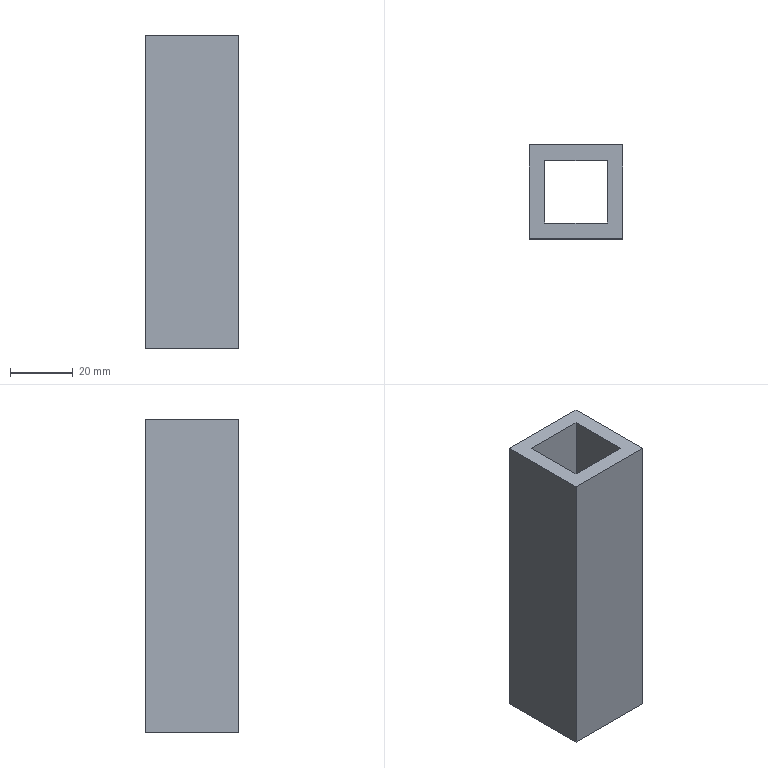Part | NX | features solid 2 | 1 solid | 10 faces | box 30 x 30 x 100 mm | volume 50000 mm3 | plane 10
STEP:
#1=CARTESIAN_POINT('',(-205.,215.,-80.));
#2=VERTEX_POINT('',#1);
#3=CARTESIAN_POINT('',(-175.,215.,-80.));
#4=VERTEX_POINT('',#3);
#5=CARTESIAN_POINT('',(-605.,215.,-80.));
#6=DIRECTION('',(-1.,0.,0.));
#7=VECTOR('',#6,1000.);
#8=LINE('',#5,#7);
#9=EDGE_CURVE('',#2,#4,#8,.F.);
#10=ORIENTED_EDGE('',*,*,#9,.F.);
#11=CARTESIAN_POINT('',(-205.,215.,-180.));
#12=VERTEX_POINT('',#11);
#13=CARTESIAN_POINT('',(-205.,215.,-125.));
#14=DIRECTION('',(0.,0.,1.));
#15=VECTOR('',#14,1000.);
#16=LINE('',#13,#15);
#17=EDGE_CURVE('',#2,#12,#16,.F.);
#18=ORIENTED_EDGE('',*,*,#17,.T.);
#19=CARTESIAN_POINT('',(-175.,215.,-180.));
#20=VERTEX_POINT('',#19);
#21=CARTESIAN_POINT('',(-605.,215.,-180.));
#22=DIRECTION('',(-1.,0.,0.));
#23=VECTOR('',#22,1000.);
#24=LINE('',#21,#23);
#25=EDGE_CURVE('',#20,#12,#24,.T.);
#26=ORIENTED_EDGE('',*,*,#25,.F.);
#27=CARTESIAN_POINT('',(-175.,215.,-125.));
#28=DIRECTION('',(0.,0.,1.));
#29=VECTOR('',#28,1000.);
#30=LINE('',#27,#29);
#31=EDGE_CURVE('',#4,#20,#30,.F.);
#32=ORIENTED_EDGE('',*,*,#31,.F.);
#33=EDGE_LOOP('',(#10,#18,#26,#32));
#34=FACE_BOUND('',#33,.T.);
#35=CARTESIAN_POINT('',(-605.,215.,-125.));
#36=DIRECTION('',(0.,1.,0.));
#37=DIRECTION('',(0.,0.,-1.));
#38=AXIS2_PLACEMENT_3D('',#35,#36,#37);
#39=PLANE('',#38);
#40=ADVANCED_FACE('',(#34),#39,.F.);
#41=CARTESIAN_POINT('',(-205.,245.,-80.));
#42=VERTEX_POINT('',#41);
#43=CARTESIAN_POINT('',(-205.,245.,-180.));
#44=VERTEX_POINT('',#43);
#45=CARTESIAN_POINT('',(-205.,245.,-125.));
#46=DIRECTION('',(0.,0.,1.));
#47=VECTOR('',#46,1000.);
#48=LINE('',#45,#47);
#49=EDGE_CURVE('',#42,#44,#48,.F.);
#50=ORIENTED_EDGE('',*,*,#49,.F.);
#51=CARTESIAN_POINT('',(-175.,245.,-80.));
#52=VERTEX_POINT('',#51);
#53=CARTESIAN_POINT('',(-605.,245.,-80.));
#54=DIRECTION('',(-1.,0.,0.));
#55=VECTOR('',#54,1000.);
#56=LINE('',#53,#55);
#57=EDGE_CURVE('',#42,#52,#56,.F.);
#58=ORIENTED_EDGE('',*,*,#57,.T.);
#59=CARTESIAN_POINT('',(-175.,245.,-180.));
#60=VERTEX_POINT('',#59);
#61=CARTESIAN_POINT('',(-175.,245.,-125.));
#62=DIRECTION('',(0.,0.,1.));
#63=VECTOR('',#62,1000.);
#64=LINE('',#61,#63);
#65=EDGE_CURVE('',#52,#60,#64,.F.);
#66=ORIENTED_EDGE('',*,*,#65,.T.);
#67=CARTESIAN_POINT('',(-605.,245.,-180.));
#68=DIRECTION('',(-1.,0.,0.));
#69=VECTOR('',#68,1000.);
#70=LINE('',#67,#69);
#71=EDGE_CURVE('',#60,#44,#70,.T.);
#72=ORIENTED_EDGE('',*,*,#71,.T.);
#73=EDGE_LOOP('',(#50,#58,#66,#72));
#74=FACE_BOUND('',#73,.T.);
#75=CARTESIAN_POINT('',(-605.,245.,-125.));
#76=DIRECTION('',(0.,1.,0.));
#77=DIRECTION('',(0.,0.,-1.));
#78=AXIS2_PLACEMENT_3D('',#75,#76,#77);
#79=PLANE('',#78);
#80=ADVANCED_FACE('',(#74),#79,.T.);
#81=CARTESIAN_POINT('',(-205.,245.,-80.));
#82=DIRECTION('',(0.,-1.,0.));
#83=VECTOR('',#82,1000.);
#84=LINE('',#81,#83);
#85=EDGE_CURVE('',#42,#2,#84,.T.);
#86=ORIENTED_EDGE('',*,*,#85,.F.);
#87=ORIENTED_EDGE('',*,*,#49,.T.);
#88=CARTESIAN_POINT('',(-205.,295.,-180.));
#89=DIRECTION('',(0.,1.,0.));
#90=VECTOR('',#89,1000.);
#91=LINE('',#88,#90);
#92=EDGE_CURVE('',#44,#12,#91,.F.);
#93=ORIENTED_EDGE('',*,*,#92,.T.);
#94=ORIENTED_EDGE('',*,*,#17,.F.);
#95=EDGE_LOOP('',(#86,#87,#93,#94));
#96=FACE_BOUND('',#95,.T.);
#97=CARTESIAN_POINT('',(-205.,245.,-125.));
#98=DIRECTION('',(-1.,0.,0.));
#99=DIRECTION('',(0.,0.,1.));
#100=AXIS2_PLACEMENT_3D('',#97,#98,#99);
#101=PLANE('',#100);
#102=ADVANCED_FACE('',(#96),#101,.T.);
#103=ORIENTED_EDGE('',*,*,#65,.F.);
#104=CARTESIAN_POINT('',(-175.,245.,-80.));
#105=DIRECTION('',(0.,-1.,0.));
#106=VECTOR('',#105,1000.);
#107=LINE('',#104,#106);
#108=EDGE_CURVE('',#52,#4,#107,.T.);
#109=ORIENTED_EDGE('',*,*,#108,.T.);
#110=ORIENTED_EDGE('',*,*,#31,.T.);
#111=CARTESIAN_POINT('',(-175.,295.,-180.));
#112=DIRECTION('',(0.,1.,0.));
#113=VECTOR('',#112,1000.);
#114=LINE('',#111,#113);
#115=EDGE_CURVE('',#60,#20,#114,.F.);
#116=ORIENTED_EDGE('',*,*,#115,.F.);
#117=EDGE_LOOP('',(#103,#109,#110,#116));
#118=FACE_BOUND('',#117,.T.);
#119=CARTESIAN_POINT('',(-175.,245.,-125.));
#120=DIRECTION('',(-1.,0.,0.));
#121=DIRECTION('',(0.,0.,1.));
#122=AXIS2_PLACEMENT_3D('',#119,#120,#121);
#123=PLANE('',#122);
#124=ADVANCED_FACE('',(#118),#123,.F.);
#125=ORIENTED_EDGE('',*,*,#25,.T.);
#126=ORIENTED_EDGE('',*,*,#92,.F.);
#127=ORIENTED_EDGE('',*,*,#71,.F.);
#128=ORIENTED_EDGE('',*,*,#115,.T.);
#129=EDGE_LOOP('',(#125,#126,#127,#128));
#130=FACE_BOUND('',#129,.T.);
#131=CARTESIAN_POINT('',(-180.,220.,-180.));
#132=VERTEX_POINT('',#131);
#133=CARTESIAN_POINT('',(-200.,220.,-180.));
#134=VERTEX_POINT('',#133);
#135=CARTESIAN_POINT('',(-605.,220.,-180.));
#136=DIRECTION('',(-1.,0.,0.));
#137=VECTOR('',#136,1000.);
#138=LINE('',#135,#137);
#139=EDGE_CURVE('',#132,#134,#138,.T.);
#140=ORIENTED_EDGE('',*,*,#139,.F.);
#141=CARTESIAN_POINT('',(-180.,240.,-180.));
#142=VERTEX_POINT('',#141);
#143=CARTESIAN_POINT('',(-180.,295.,-180.));
#144=DIRECTION('',(0.,1.,0.));
#145=VECTOR('',#144,1000.);
#146=LINE('',#143,#145);
#147=EDGE_CURVE('',#142,#132,#146,.F.);
#148=ORIENTED_EDGE('',*,*,#147,.F.);
#149=CARTESIAN_POINT('',(-200.,240.,-180.));
#150=VERTEX_POINT('',#149);
#151=CARTESIAN_POINT('',(-605.,240.,-180.));
#152=DIRECTION('',(-1.,0.,0.));
#153=VECTOR('',#152,1000.);
#154=LINE('',#151,#153);
#155=EDGE_CURVE('',#142,#150,#154,.T.);
#156=ORIENTED_EDGE('',*,*,#155,.T.);
#157=CARTESIAN_POINT('',(-200.,295.,-180.));
#158=DIRECTION('',(0.,1.,0.));
#159=VECTOR('',#158,1000.);
#160=LINE('',#157,#159);
#161=EDGE_CURVE('',#150,#134,#160,.F.);
#162=ORIENTED_EDGE('',*,*,#161,.T.);
#163=EDGE_LOOP('',(#140,#148,#156,#162));
#164=FACE_BOUND('',#163,.T.);
#165=CARTESIAN_POINT('',(-175.,295.,-180.));
#166=DIRECTION('',(0.,0.,-1.));
#167=DIRECTION('',(-1.,0.,0.));
#168=AXIS2_PLACEMENT_3D('',#165,#166,#167);
#169=PLANE('',#168);
#170=ADVANCED_FACE('',(#130,#164),#169,.T.);
#171=CARTESIAN_POINT('',(-200.,220.,-80.));
#172=VERTEX_POINT('',#171);
#173=CARTESIAN_POINT('',(-200.,220.,-125.));
#174=DIRECTION('',(0.,0.,1.));
#175=VECTOR('',#174,1000.);
#176=LINE('',#173,#175);
#177=EDGE_CURVE('',#172,#134,#176,.F.);
#178=ORIENTED_EDGE('',*,*,#177,.F.);
#179=CARTESIAN_POINT('',(-180.,220.,-80.));
#180=VERTEX_POINT('',#179);
#181=CARTESIAN_POINT('',(-605.,220.,-80.));
#182=DIRECTION('',(-1.,0.,0.));
#183=VECTOR('',#182,1000.);
#184=LINE('',#181,#183);
#185=EDGE_CURVE('',#172,#180,#184,.F.);
#186=ORIENTED_EDGE('',*,*,#185,.T.);
#187=CARTESIAN_POINT('',(-180.,220.,-125.));
#188=DIRECTION('',(0.,0.,1.));
#189=VECTOR('',#188,1000.);
#190=LINE('',#187,#189);
#191=EDGE_CURVE('',#180,#132,#190,.F.);
#192=ORIENTED_EDGE('',*,*,#191,.T.);
#193=ORIENTED_EDGE('',*,*,#139,.T.);
#194=EDGE_LOOP('',(#178,#186,#192,#193));
#195=FACE_BOUND('',#194,.T.);
#196=CARTESIAN_POINT('',(-605.,220.,-125.));
#197=DIRECTION('',(0.,1.,0.));
#198=DIRECTION('',(0.,0.,-1.));
#199=AXIS2_PLACEMENT_3D('',#196,#197,#198);
#200=PLANE('',#199);
#201=ADVANCED_FACE('',(#195),#200,.T.);
#202=CARTESIAN_POINT('',(-200.,240.,-80.));
#203=VERTEX_POINT('',#202);
#204=CARTESIAN_POINT('',(-180.,240.,-80.));
#205=VERTEX_POINT('',#204);
#206=CARTESIAN_POINT('',(-605.,240.,-80.));
#207=DIRECTION('',(-1.,0.,0.));
#208=VECTOR('',#207,1000.);
#209=LINE('',#206,#208);
#210=EDGE_CURVE('',#203,#205,#209,.F.);
#211=ORIENTED_EDGE('',*,*,#210,.F.);
#212=CARTESIAN_POINT('',(-200.,240.,-125.));
#213=DIRECTION('',(0.,0.,1.));
#214=VECTOR('',#213,1000.);
#215=LINE('',#212,#214);
#216=EDGE_CURVE('',#203,#150,#215,.F.);
#217=ORIENTED_EDGE('',*,*,#216,.T.);
#218=ORIENTED_EDGE('',*,*,#155,.F.);
#219=CARTESIAN_POINT('',(-180.,240.,-125.));
#220=DIRECTION('',(0.,0.,1.));
#221=VECTOR('',#220,1000.);
#222=LINE('',#219,#221);
#223=EDGE_CURVE('',#205,#142,#222,.F.);
#224=ORIENTED_EDGE('',*,*,#223,.F.);
#225=EDGE_LOOP('',(#211,#217,#218,#224));
#226=FACE_BOUND('',#225,.T.);
#227=CARTESIAN_POINT('',(-605.,240.,-125.));
#228=DIRECTION('',(0.,1.,0.));
#229=DIRECTION('',(0.,0.,-1.));
#230=AXIS2_PLACEMENT_3D('',#227,#228,#229);
#231=PLANE('',#230);
#232=ADVANCED_FACE('',(#226),#231,.F.);
#233=ORIENTED_EDGE('',*,*,#216,.F.);
#234=CARTESIAN_POINT('',(-200.,245.,-80.));
#235=DIRECTION('',(0.,-1.,0.));
#236=VECTOR('',#235,1000.);
#237=LINE('',#234,#236);
#238=EDGE_CURVE('',#203,#172,#237,.T.);
#239=ORIENTED_EDGE('',*,*,#238,.T.);
#240=ORIENTED_EDGE('',*,*,#177,.T.);
#241=ORIENTED_EDGE('',*,*,#161,.F.);
#242=EDGE_LOOP('',(#233,#239,#240,#241));
#243=FACE_BOUND('',#242,.T.);
#244=CARTESIAN_POINT('',(-200.,245.,-125.));
#245=DIRECTION('',(-1.,0.,0.));
#246=DIRECTION('',(0.,0.,1.));
#247=AXIS2_PLACEMENT_3D('',#244,#245,#246);
#248=PLANE('',#247);
#249=ADVANCED_FACE('',(#243),#248,.F.);
#250=CARTESIAN_POINT('',(-180.,245.,-80.));
#251=DIRECTION('',(0.,-1.,0.));
#252=VECTOR('',#251,1000.);
#253=LINE('',#250,#252);
#254=EDGE_CURVE('',#205,#180,#253,.T.);
#255=ORIENTED_EDGE('',*,*,#254,.F.);
#256=ORIENTED_EDGE('',*,*,#223,.T.);
#257=ORIENTED_EDGE('',*,*,#147,.T.);
#258=ORIENTED_EDGE('',*,*,#191,.F.);
#259=EDGE_LOOP('',(#255,#256,#257,#258));
#260=FACE_BOUND('',#259,.T.);
#261=CARTESIAN_POINT('',(-180.,245.,-125.));
#262=DIRECTION('',(-1.,0.,0.));
#263=DIRECTION('',(0.,0.,1.));
#264=AXIS2_PLACEMENT_3D('',#261,#262,#263);
#265=PLANE('',#264);
#266=ADVANCED_FACE('',(#260),#265,.T.);
#267=ORIENTED_EDGE('',*,*,#210,.T.);
#268=ORIENTED_EDGE('',*,*,#254,.T.);
#269=ORIENTED_EDGE('',*,*,#185,.F.);
#270=ORIENTED_EDGE('',*,*,#238,.F.);
#271=EDGE_LOOP('',(#267,#268,#269,#270));
#272=FACE_BOUND('',#271,.T.);
#273=ORIENTED_EDGE('',*,*,#85,.T.);
#274=ORIENTED_EDGE('',*,*,#9,.T.);
#275=ORIENTED_EDGE('',*,*,#108,.F.);
#276=ORIENTED_EDGE('',*,*,#57,.F.);
#277=EDGE_LOOP('',(#273,#274,#275,#276));
#278=FACE_BOUND('',#277,.T.);
#279=CARTESIAN_POINT('',(-140.,-165.,-80.));
#280=DIRECTION('',(0.,0.,-1.));
#281=DIRECTION('',(-1.,0.,0.));
#282=AXIS2_PLACEMENT_3D('',#279,#280,#281);
#283=PLANE('',#282);
#284=ADVANCED_FACE('',(#272,#278),#283,.F.);
#285=CLOSED_SHELL('',(#40,#80,#102,#124,#170,#201,#232,#249,#266,#284));
#286=MANIFOLD_SOLID_BREP('',#285);
#287=(LENGTH_UNIT()NAMED_UNIT(*)SI_UNIT(.MILLI.,.METRE.));
#288=UNCERTAINTY_MEASURE_WITH_UNIT(LENGTH_MEASURE(0.00001),#287,'','');
#289=(NAMED_UNIT(*)PLANE_ANGLE_UNIT()SI_UNIT($,.RADIAN.));
#290=(NAMED_UNIT(*)SI_UNIT($,.STERADIAN.)SOLID_ANGLE_UNIT());
#291=(GEOMETRIC_REPRESENTATION_CONTEXT(3)GLOBAL_UNCERTAINTY_ASSIGNED_CONTEXT((#288))GLOBAL_UNIT_ASSIGNED_CONTEXT((#287,#289,#290))REPRESENTATION_CONTEXT('',''));
#292=ADVANCED_BREP_SHAPE_REPRESENTATION('',(#286),#291);